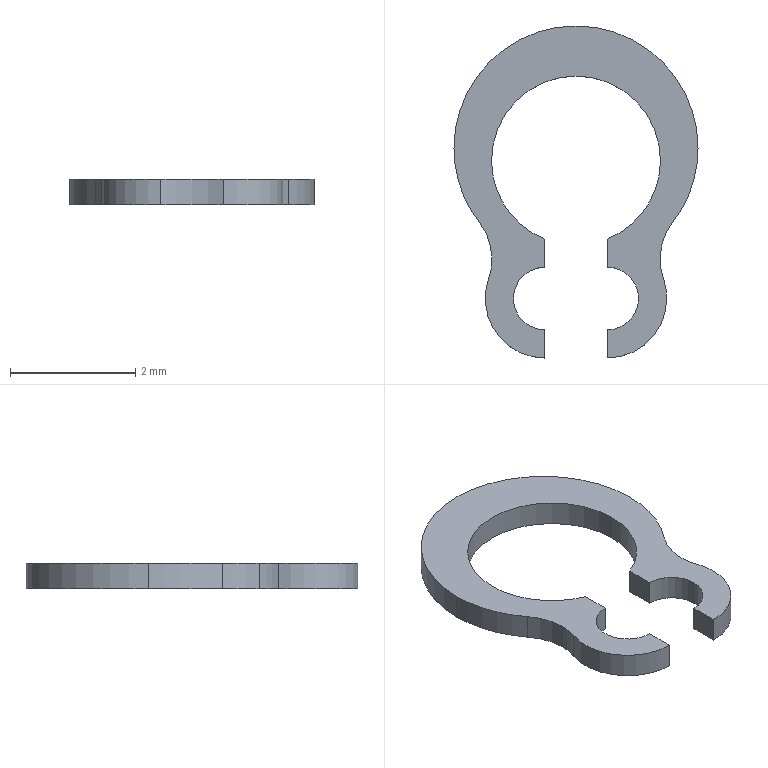Part | SolidWorks | features Boss 1 | 1 solid | 21 faces | box 3.9 x 5.304 x 0.4 mm | volume 3.093 mm3 | cylinder 15 | plane 6 | commonest cylinder face diameters 1.9 x6 1 x3 2.7 x3 3.9 x3
STEP:
#1=CARTESIAN_POINT('',(-0.5,-1.454,-0.4));
#2=VERTEX_POINT('',#1);
#3=CARTESIAN_POINT('',(-1.35,-0.2,-0.4));
#4=VERTEX_POINT('',#3);
#5=CARTESIAN_POINT('',(0.,-0.2,-0.4));
#6=DIRECTION('',(0.,0.,-1.));
#7=DIRECTION('',(1.,0.,0.));
#8=AXIS2_PLACEMENT_3D('',#5,#6,#7);
#9=CIRCLE('',#8,1.35);
#10=EDGE_CURVE('',#2,#4,#9,.T.);
#11=ORIENTED_EDGE('',*,*,#10,.T.);
#12=CARTESIAN_POINT('',(-1.35,-0.2,0.));
#13=VERTEX_POINT('',#12);
#14=CARTESIAN_POINT('',(-1.35,-0.2,-0.4));
#15=DIRECTION('',(0.,0.,1.));
#16=VECTOR('',#15,1000.);
#17=LINE('',#14,#16);
#18=EDGE_CURVE('',#4,#13,#17,.T.);
#19=ORIENTED_EDGE('',*,*,#18,.T.);
#20=CARTESIAN_POINT('',(-0.5,-1.454,0.));
#21=VERTEX_POINT('',#20);
#22=CARTESIAN_POINT('',(0.,-0.2,0.));
#23=DIRECTION('',(0.,0.,-1.));
#24=DIRECTION('',(1.,0.,0.));
#25=AXIS2_PLACEMENT_3D('',#22,#23,#24);
#26=CIRCLE('',#25,1.35);
#27=EDGE_CURVE('',#21,#13,#26,.T.);
#28=ORIENTED_EDGE('',*,*,#27,.F.);
#29=CARTESIAN_POINT('',(-0.5,-1.454,-0.4));
#30=DIRECTION('',(0.,0.,1.));
#31=VECTOR('',#30,1000.);
#32=LINE('',#29,#31);
#33=EDGE_CURVE('',#2,#21,#32,.T.);
#34=ORIENTED_EDGE('',*,*,#33,.F.);
#35=EDGE_LOOP('',(#11,#19,#28,#34));
#36=FACE_OUTER_BOUND('',#35,.T.);
#37=CARTESIAN_POINT('',(0.,-0.2,-0.4));
#38=DIRECTION('',(0.,0.,1.));
#39=DIRECTION('',(1.,0.,0.));
#40=AXIS2_PLACEMENT_3D('',#37,#38,#39);
#41=CYLINDRICAL_SURFACE('',#40,1.35);
#42=ADVANCED_FACE('',(#36),#41,.F.);
#43=ORIENTED_EDGE('',*,*,#18,.F.);
#44=CARTESIAN_POINT('',(1.35,-0.2,-0.4));
#45=VERTEX_POINT('',#44);
#46=CARTESIAN_POINT('',(0.,-0.2,-0.4));
#47=DIRECTION('',(0.,0.,-1.));
#48=DIRECTION('',(1.,0.,0.));
#49=AXIS2_PLACEMENT_3D('',#46,#47,#48);
#50=CIRCLE('',#49,1.35);
#51=EDGE_CURVE('',#4,#45,#50,.T.);
#52=ORIENTED_EDGE('',*,*,#51,.T.);
#53=CARTESIAN_POINT('',(1.35,-0.2,0.));
#54=VERTEX_POINT('',#53);
#55=CARTESIAN_POINT('',(1.35,-0.2,-0.4));
#56=DIRECTION('',(0.,0.,1.));
#57=VECTOR('',#56,1000.);
#58=LINE('',#55,#57);
#59=EDGE_CURVE('',#45,#54,#58,.T.);
#60=ORIENTED_EDGE('',*,*,#59,.T.);
#61=CARTESIAN_POINT('',(0.,-0.2,0.));
#62=DIRECTION('',(0.,0.,-1.));
#63=DIRECTION('',(1.,0.,0.));
#64=AXIS2_PLACEMENT_3D('',#61,#62,#63);
#65=CIRCLE('',#64,1.35);
#66=EDGE_CURVE('',#13,#54,#65,.T.);
#67=ORIENTED_EDGE('',*,*,#66,.F.);
#68=EDGE_LOOP('',(#43,#52,#60,#67));
#69=FACE_OUTER_BOUND('',#68,.T.);
#70=CARTESIAN_POINT('',(0.,-0.2,-0.4));
#71=DIRECTION('',(0.,0.,1.));
#72=DIRECTION('',(1.,0.,0.));
#73=AXIS2_PLACEMENT_3D('',#70,#71,#72);
#74=CYLINDRICAL_SURFACE('',#73,1.35);
#75=ADVANCED_FACE('',(#69),#74,.F.);
#76=CARTESIAN_POINT('',(0.5,-1.904,-0.4));
#77=VERTEX_POINT('',#76);
#78=CARTESIAN_POINT('',(1.,-2.404,-0.4));
#79=VERTEX_POINT('',#78);
#80=CARTESIAN_POINT('',(0.5,-2.404,-0.4));
#81=DIRECTION('',(0.,0.,-1.));
#82=DIRECTION('',(-1.,0.,0.));
#83=AXIS2_PLACEMENT_3D('',#80,#81,#82);
#84=CIRCLE('',#83,0.5);
#85=EDGE_CURVE('',#77,#79,#84,.T.);
#86=ORIENTED_EDGE('',*,*,#85,.T.);
#87=CARTESIAN_POINT('',(1.,-2.404,0.));
#88=VERTEX_POINT('',#87);
#89=CARTESIAN_POINT('',(1.,-2.404,-0.4));
#90=DIRECTION('',(0.,0.,1.));
#91=VECTOR('',#90,1000.);
#92=LINE('',#89,#91);
#93=EDGE_CURVE('',#79,#88,#92,.T.);
#94=ORIENTED_EDGE('',*,*,#93,.T.);
#95=CARTESIAN_POINT('',(0.5,-1.904,0.));
#96=VERTEX_POINT('',#95);
#97=CARTESIAN_POINT('',(0.5,-2.404,0.));
#98=DIRECTION('',(0.,0.,-1.));
#99=DIRECTION('',(-1.,0.,0.));
#100=AXIS2_PLACEMENT_3D('',#97,#98,#99);
#101=CIRCLE('',#100,0.5);
#102=EDGE_CURVE('',#96,#88,#101,.T.);
#103=ORIENTED_EDGE('',*,*,#102,.F.);
#104=CARTESIAN_POINT('',(0.5,-1.904,-0.4));
#105=DIRECTION('',(0.,0.,1.));
#106=VECTOR('',#105,1000.);
#107=LINE('',#104,#106);
#108=EDGE_CURVE('',#77,#96,#107,.T.);
#109=ORIENTED_EDGE('',*,*,#108,.F.);
#110=EDGE_LOOP('',(#86,#94,#103,#109));
#111=FACE_OUTER_BOUND('',#110,.T.);
#112=CARTESIAN_POINT('',(0.5,-2.404,-0.4));
#113=DIRECTION('',(0.,0.,1.));
#114=DIRECTION('',(1.,0.,0.));
#115=AXIS2_PLACEMENT_3D('',#112,#113,#114);
#116=CYLINDRICAL_SURFACE('',#115,0.5);
#117=ADVANCED_FACE('',(#111),#116,.F.);
#118=CARTESIAN_POINT('',(0.5,-3.354,-0.4));
#119=VERTEX_POINT('',#118);
#120=CARTESIAN_POINT('',(1.45,-2.404,-0.4));
#121=VERTEX_POINT('',#120);
#122=CARTESIAN_POINT('',(0.5,-2.404,-0.4));
#123=DIRECTION('',(0.,0.,1.));
#124=DIRECTION('',(1.,0.,0.));
#125=AXIS2_PLACEMENT_3D('',#122,#123,#124);
#126=CIRCLE('',#125,0.95);
#127=EDGE_CURVE('',#119,#121,#126,.T.);
#128=ORIENTED_EDGE('',*,*,#127,.T.);
#129=CARTESIAN_POINT('',(1.45,-2.404,0.));
#130=VERTEX_POINT('',#129);
#131=CARTESIAN_POINT('',(1.45,-2.404,-0.4));
#132=DIRECTION('',(0.,0.,1.));
#133=VECTOR('',#132,1000.);
#134=LINE('',#131,#133);
#135=EDGE_CURVE('',#121,#130,#134,.T.);
#136=ORIENTED_EDGE('',*,*,#135,.T.);
#137=CARTESIAN_POINT('',(0.5,-3.354,0.));
#138=VERTEX_POINT('',#137);
#139=CARTESIAN_POINT('',(0.5,-2.404,0.));
#140=DIRECTION('',(0.,0.,1.));
#141=DIRECTION('',(1.,0.,0.));
#142=AXIS2_PLACEMENT_3D('',#139,#140,#141);
#143=CIRCLE('',#142,0.95);
#144=EDGE_CURVE('',#138,#130,#143,.T.);
#145=ORIENTED_EDGE('',*,*,#144,.F.);
#146=CARTESIAN_POINT('',(0.5,-3.354,-0.4));
#147=DIRECTION('',(0.,0.,1.));
#148=VECTOR('',#147,1000.);
#149=LINE('',#146,#148);
#150=EDGE_CURVE('',#119,#138,#149,.T.);
#151=ORIENTED_EDGE('',*,*,#150,.F.);
#152=EDGE_LOOP('',(#128,#136,#145,#151));
#153=FACE_OUTER_BOUND('',#152,.T.);
#154=CARTESIAN_POINT('',(0.5,-2.404,-0.4));
#155=DIRECTION('',(0.,0.,1.));
#156=DIRECTION('',(1.,0.,0.));
#157=AXIS2_PLACEMENT_3D('',#154,#155,#156);
#158=CYLINDRICAL_SURFACE('',#157,0.95);
#159=ADVANCED_FACE('',(#153),#158,.T.);
#160=CARTESIAN_POINT('',(1.95,0.,-0.4));
#161=VERTEX_POINT('',#160);
#162=CARTESIAN_POINT('',(-1.95,0.,-0.4));
#163=VERTEX_POINT('',#162);
#164=CARTESIAN_POINT('',(0.,0.,-0.4));
#165=DIRECTION('',(0.,0.,1.));
#166=DIRECTION('',(1.,0.,0.));
#167=AXIS2_PLACEMENT_3D('',#164,#165,#166);
#168=CIRCLE('',#167,1.95);
#169=EDGE_CURVE('',#161,#163,#168,.T.);
#170=ORIENTED_EDGE('',*,*,#169,.T.);
#171=CARTESIAN_POINT('',(-1.95,0.,0.));
#172=VERTEX_POINT('',#171);
#173=CARTESIAN_POINT('',(-1.95,0.,-0.4));
#174=DIRECTION('',(0.,0.,1.));
#175=VECTOR('',#174,1000.);
#176=LINE('',#173,#175);
#177=EDGE_CURVE('',#163,#172,#176,.T.);
#178=ORIENTED_EDGE('',*,*,#177,.T.);
#179=CARTESIAN_POINT('',(1.95,0.,0.));
#180=VERTEX_POINT('',#179);
#181=CARTESIAN_POINT('',(0.,0.,0.));
#182=DIRECTION('',(0.,0.,1.));
#183=DIRECTION('',(1.,0.,0.));
#184=AXIS2_PLACEMENT_3D('',#181,#182,#183);
#185=CIRCLE('',#184,1.95);
#186=EDGE_CURVE('',#180,#172,#185,.T.);
#187=ORIENTED_EDGE('',*,*,#186,.F.);
#188=CARTESIAN_POINT('',(1.95,0.,-0.4));
#189=DIRECTION('',(0.,0.,1.));
#190=VECTOR('',#189,1000.);
#191=LINE('',#188,#190);
#192=EDGE_CURVE('',#161,#180,#191,.T.);
#193=ORIENTED_EDGE('',*,*,#192,.F.);
#194=EDGE_LOOP('',(#170,#178,#187,#193));
#195=FACE_OUTER_BOUND('',#194,.T.);
#196=CARTESIAN_POINT('',(0.,0.,-0.4));
#197=DIRECTION('',(0.,0.,1.));
#198=DIRECTION('',(1.,0.,0.));
#199=AXIS2_PLACEMENT_3D('',#196,#197,#198);
#200=CYLINDRICAL_SURFACE('',#199,1.95);
#201=ADVANCED_FACE('',(#195),#200,.T.);
#202=CARTESIAN_POINT('',(1.542,-1.194,-0.4));
#203=VERTEX_POINT('',#202);
#204=CARTESIAN_POINT('',(0.,0.,-0.4));
#205=DIRECTION('',(0.,0.,1.));
#206=DIRECTION('',(1.,0.,0.));
#207=AXIS2_PLACEMENT_3D('',#204,#205,#206);
#208=CIRCLE('',#207,1.95);
#209=EDGE_CURVE('',#203,#161,#208,.T.);
#210=ORIENTED_EDGE('',*,*,#209,.T.);
#211=ORIENTED_EDGE('',*,*,#192,.T.);
#212=CARTESIAN_POINT('',(1.542,-1.194,0.));
#213=VERTEX_POINT('',#212);
#214=CARTESIAN_POINT('',(0.,0.,0.));
#215=DIRECTION('',(0.,0.,1.));
#216=DIRECTION('',(1.,0.,0.));
#217=AXIS2_PLACEMENT_3D('',#214,#215,#216);
#218=CIRCLE('',#217,1.95);
#219=EDGE_CURVE('',#213,#180,#218,.T.);
#220=ORIENTED_EDGE('',*,*,#219,.F.);
#221=CARTESIAN_POINT('',(1.542,-1.194,-0.4));
#222=DIRECTION('',(0.,0.,1.));
#223=VECTOR('',#222,1000.);
#224=LINE('',#221,#223);
#225=EDGE_CURVE('',#203,#213,#224,.T.);
#226=ORIENTED_EDGE('',*,*,#225,.F.);
#227=EDGE_LOOP('',(#210,#211,#220,#226));
#228=FACE_OUTER_BOUND('',#227,.T.);
#229=CARTESIAN_POINT('',(0.,0.,-0.4));
#230=DIRECTION('',(0.,0.,1.));
#231=DIRECTION('',(1.,0.,0.));
#232=AXIS2_PLACEMENT_3D('',#229,#230,#231);
#233=CYLINDRICAL_SURFACE('',#232,1.95);
#234=ADVANCED_FACE('',(#228),#233,.T.);
#235=CARTESIAN_POINT('',(-1.542,-1.194,-0.4));
#236=VERTEX_POINT('',#235);
#237=CARTESIAN_POINT('',(-1.343,-1.775,-0.4));
#238=VERTEX_POINT('',#237);
#239=CARTESIAN_POINT('',(-2.293,-1.775,-0.4));
#240=DIRECTION('',(0.,0.,-1.));
#241=DIRECTION('',(-1.,0.,0.));
#242=AXIS2_PLACEMENT_3D('',#239,#240,#241);
#243=CIRCLE('',#242,0.95);
#244=EDGE_CURVE('',#236,#238,#243,.T.);
#245=ORIENTED_EDGE('',*,*,#244,.T.);
#246=CARTESIAN_POINT('',(-1.343,-1.775,0.));
#247=VERTEX_POINT('',#246);
#248=CARTESIAN_POINT('',(-1.343,-1.775,-0.4));
#249=DIRECTION('',(0.,0.,1.));
#250=VECTOR('',#249,1000.);
#251=LINE('',#248,#250);
#252=EDGE_CURVE('',#238,#247,#251,.T.);
#253=ORIENTED_EDGE('',*,*,#252,.T.);
#254=CARTESIAN_POINT('',(-1.542,-1.194,0.));
#255=VERTEX_POINT('',#254);
#256=CARTESIAN_POINT('',(-2.293,-1.775,0.));
#257=DIRECTION('',(0.,0.,-1.));
#258=DIRECTION('',(-1.,0.,0.));
#259=AXIS2_PLACEMENT_3D('',#256,#257,#258);
#260=CIRCLE('',#259,0.95);
#261=EDGE_CURVE('',#255,#247,#260,.T.);
#262=ORIENTED_EDGE('',*,*,#261,.F.);
#263=CARTESIAN_POINT('',(-1.542,-1.194,-0.4));
#264=DIRECTION('',(0.,0.,1.));
#265=VECTOR('',#264,1000.);
#266=LINE('',#263,#265);
#267=EDGE_CURVE('',#236,#255,#266,.T.);
#268=ORIENTED_EDGE('',*,*,#267,.F.);
#269=EDGE_LOOP('',(#245,#253,#262,#268));
#270=FACE_OUTER_BOUND('',#269,.T.);
#271=CARTESIAN_POINT('',(-2.293,-1.775,-0.4));
#272=DIRECTION('',(0.,0.,1.));
#273=DIRECTION('',(1.,0.,0.));
#274=AXIS2_PLACEMENT_3D('',#271,#272,#273);
#275=CYLINDRICAL_SURFACE('',#274,0.95);
#276=ADVANCED_FACE('',(#270),#275,.F.);
#277=CARTESIAN_POINT('',(-0.5,-2.904,0.));
#278=VERTEX_POINT('',#277);
#279=CARTESIAN_POINT('',(-0.5,-1.904,0.));
#280=VERTEX_POINT('',#279);
#281=CARTESIAN_POINT('',(-0.5,-2.404,0.));
#282=DIRECTION('',(0.,0.,-1.));
#283=DIRECTION('',(1.,0.,0.));
#284=AXIS2_PLACEMENT_3D('',#281,#282,#283);
#285=CIRCLE('',#284,0.5);
#286=EDGE_CURVE('',#278,#280,#285,.T.);
#287=ORIENTED_EDGE('',*,*,#286,.F.);
#288=CARTESIAN_POINT('',(-0.5,-2.904,-0.4));
#289=VERTEX_POINT('',#288);
#290=CARTESIAN_POINT('',(-0.5,-2.904,-0.4));
#291=DIRECTION('',(0.,0.,1.));
#292=VECTOR('',#291,1000.);
#293=LINE('',#290,#292);
#294=EDGE_CURVE('',#289,#278,#293,.T.);
#295=ORIENTED_EDGE('',*,*,#294,.F.);
#296=CARTESIAN_POINT('',(-0.5,-1.904,-0.4));
#297=VERTEX_POINT('',#296);
#298=CARTESIAN_POINT('',(-0.5,-2.404,-0.4));
#299=DIRECTION('',(0.,0.,-1.));
#300=DIRECTION('',(1.,0.,0.));
#301=AXIS2_PLACEMENT_3D('',#298,#299,#300);
#302=CIRCLE('',#301,0.5);
#303=EDGE_CURVE('',#289,#297,#302,.T.);
#304=ORIENTED_EDGE('',*,*,#303,.T.);
#305=CARTESIAN_POINT('',(-0.5,-1.904,-0.4));
#306=DIRECTION('',(0.,0.,1.));
#307=VECTOR('',#306,1000.);
#308=LINE('',#305,#307);
#309=EDGE_CURVE('',#297,#280,#308,.T.);
#310=ORIENTED_EDGE('',*,*,#309,.T.);
#311=EDGE_LOOP('',(#287,#295,#304,#310));
#312=FACE_OUTER_BOUND('',#311,.T.);
#313=CARTESIAN_POINT('',(-0.5,-2.404,-0.4));
#314=DIRECTION('',(0.,0.,1.));
#315=DIRECTION('',(1.,0.,0.));
#316=AXIS2_PLACEMENT_3D('',#313,#314,#315);
#317=CYLINDRICAL_SURFACE('',#316,0.5);
#318=ADVANCED_FACE('',(#312),#317,.F.);
#319=CARTESIAN_POINT('',(-0.5,-3.354,0.));
#320=VERTEX_POINT('',#319);
#321=CARTESIAN_POINT('',(-0.5,-2.904,0.));
#322=DIRECTION('',(0.,1.,0.));
#323=VECTOR('',#322,1000.);
#324=LINE('',#321,#323);
#325=EDGE_CURVE('',#320,#278,#324,.T.);
#326=ORIENTED_EDGE('',*,*,#325,.F.);
#327=CARTESIAN_POINT('',(-0.5,-3.354,-0.4));
#328=VERTEX_POINT('',#327);
#329=CARTESIAN_POINT('',(-0.5,-3.354,-0.4));
#330=DIRECTION('',(0.,0.,1.));
#331=VECTOR('',#330,1000.);
#332=LINE('',#329,#331);
#333=EDGE_CURVE('',#328,#320,#332,.T.);
#334=ORIENTED_EDGE('',*,*,#333,.F.);
#335=CARTESIAN_POINT('',(-0.5,-2.904,-0.4));
#336=DIRECTION('',(0.,1.,0.));
#337=VECTOR('',#336,1000.);
#338=LINE('',#335,#337);
#339=EDGE_CURVE('',#328,#289,#338,.T.);
#340=ORIENTED_EDGE('',*,*,#339,.T.);
#341=ORIENTED_EDGE('',*,*,#294,.T.);
#342=EDGE_LOOP('',(#326,#334,#340,#341));
#343=FACE_OUTER_BOUND('',#342,.T.);
#344=CARTESIAN_POINT('',(-0.5,-2.904,-0.4));
#345=DIRECTION('',(1.,0.,0.));
#346=DIRECTION('',(0.,0.,-1.));
#347=AXIS2_PLACEMENT_3D('',#344,#345,#346);
#348=PLANE('',#347);
#349=ADVANCED_FACE('',(#343),#348,.T.);
#350=CARTESIAN_POINT('',(-1.397,-2.09,0.));
#351=VERTEX_POINT('',#350);
#352=CARTESIAN_POINT('',(-0.5,-2.404,0.));
#353=DIRECTION('',(0.,0.,1.));
#354=DIRECTION('',(-1.,0.,0.));
#355=AXIS2_PLACEMENT_3D('',#352,#353,#354);
#356=CIRCLE('',#355,0.95);
#357=EDGE_CURVE('',#351,#320,#356,.T.);
#358=ORIENTED_EDGE('',*,*,#357,.F.);
#359=CARTESIAN_POINT('',(-1.397,-2.09,-0.4));
#360=VERTEX_POINT('',#359);
#361=CARTESIAN_POINT('',(-1.397,-2.09,-0.4));
#362=DIRECTION('',(0.,0.,1.));
#363=VECTOR('',#362,1000.);
#364=LINE('',#361,#363);
#365=EDGE_CURVE('',#360,#351,#364,.T.);
#366=ORIENTED_EDGE('',*,*,#365,.F.);
#367=CARTESIAN_POINT('',(-0.5,-2.404,-0.4));
#368=DIRECTION('',(0.,0.,1.));
#369=DIRECTION('',(-1.,0.,0.));
#370=AXIS2_PLACEMENT_3D('',#367,#368,#369);
#371=CIRCLE('',#370,0.95);
#372=EDGE_CURVE('',#360,#328,#371,.T.);
#373=ORIENTED_EDGE('',*,*,#372,.T.);
#374=ORIENTED_EDGE('',*,*,#333,.T.);
#375=EDGE_LOOP('',(#358,#366,#373,#374));
#376=FACE_OUTER_BOUND('',#375,.T.);
#377=CARTESIAN_POINT('',(-0.5,-2.404,-0.4));
#378=DIRECTION('',(0.,0.,1.));
#379=DIRECTION('',(1.,0.,0.));
#380=AXIS2_PLACEMENT_3D('',#377,#378,#379);
#381=CYLINDRICAL_SURFACE('',#380,0.95);
#382=ADVANCED_FACE('',(#376),#381,.T.);
#383=ORIENTED_EDGE('',*,*,#252,.F.);
#384=CARTESIAN_POINT('',(-2.293,-1.775,-0.4));
#385=DIRECTION('',(0.,0.,-1.));
#386=DIRECTION('',(-1.,0.,0.));
#387=AXIS2_PLACEMENT_3D('',#384,#385,#386);
#388=CIRCLE('',#387,0.95);
#389=EDGE_CURVE('',#238,#360,#388,.T.);
#390=ORIENTED_EDGE('',*,*,#389,.T.);
#391=ORIENTED_EDGE('',*,*,#365,.T.);
#392=CARTESIAN_POINT('',(-2.293,-1.775,0.));
#393=DIRECTION('',(0.,0.,-1.));
#394=DIRECTION('',(-1.,0.,0.));
#395=AXIS2_PLACEMENT_3D('',#392,#393,#394);
#396=CIRCLE('',#395,0.95);
#397=EDGE_CURVE('',#247,#351,#396,.T.);
#398=ORIENTED_EDGE('',*,*,#397,.F.);
#399=EDGE_LOOP('',(#383,#390,#391,#398));
#400=FACE_OUTER_BOUND('',#399,.T.);
#401=CARTESIAN_POINT('',(-2.293,-1.775,-0.4));
#402=DIRECTION('',(0.,0.,1.));
#403=DIRECTION('',(1.,0.,0.));
#404=AXIS2_PLACEMENT_3D('',#401,#402,#403);
#405=CYLINDRICAL_SURFACE('',#404,0.95);
#406=ADVANCED_FACE('',(#400),#405,.F.);
#407=ORIENTED_EDGE('',*,*,#177,.F.);
#408=CARTESIAN_POINT('',(0.,0.,-0.4));
#409=DIRECTION('',(0.,0.,1.));
#410=DIRECTION('',(1.,0.,0.));
#411=AXIS2_PLACEMENT_3D('',#408,#409,#410);
#412=CIRCLE('',#411,1.95);
#413=EDGE_CURVE('',#163,#236,#412,.T.);
#414=ORIENTED_EDGE('',*,*,#413,.T.);
#415=ORIENTED_EDGE('',*,*,#267,.T.);
#416=CARTESIAN_POINT('',(0.,0.,0.));
#417=DIRECTION('',(0.,0.,1.));
#418=DIRECTION('',(1.,0.,0.));
#419=AXIS2_PLACEMENT_3D('',#416,#417,#418);
#420=CIRCLE('',#419,1.95);
#421=EDGE_CURVE('',#172,#255,#420,.T.);
#422=ORIENTED_EDGE('',*,*,#421,.F.);
#423=EDGE_LOOP('',(#407,#414,#415,#422));
#424=FACE_OUTER_BOUND('',#423,.T.);
#425=CARTESIAN_POINT('',(0.,0.,-0.4));
#426=DIRECTION('',(0.,0.,1.));
#427=DIRECTION('',(1.,0.,0.));
#428=AXIS2_PLACEMENT_3D('',#425,#426,#427);
#429=CYLINDRICAL_SURFACE('',#428,1.95);
#430=ADVANCED_FACE('',(#424),#429,.T.);
#431=CARTESIAN_POINT('',(1.397,-2.09,0.));
#432=VERTEX_POINT('',#431);
#433=CARTESIAN_POINT('',(2.293,-1.775,0.));
#434=DIRECTION('',(0.,0.,-1.));
#435=DIRECTION('',(1.,0.,0.));
#436=AXIS2_PLACEMENT_3D('',#433,#434,#435);
#437=CIRCLE('',#436,0.95);
#438=EDGE_CURVE('',#432,#213,#437,.T.);
#439=ORIENTED_EDGE('',*,*,#438,.F.);
#440=CARTESIAN_POINT('',(1.397,-2.09,-0.4));
#441=VERTEX_POINT('',#440);
#442=CARTESIAN_POINT('',(1.397,-2.09,-0.4));
#443=DIRECTION('',(0.,0.,1.));
#444=VECTOR('',#443,1000.);
#445=LINE('',#442,#444);
#446=EDGE_CURVE('',#441,#432,#445,.T.);
#447=ORIENTED_EDGE('',*,*,#446,.F.);
#448=CARTESIAN_POINT('',(2.293,-1.775,-0.4));
#449=DIRECTION('',(0.,0.,-1.));
#450=DIRECTION('',(1.,0.,0.));
#451=AXIS2_PLACEMENT_3D('',#448,#449,#450);
#452=CIRCLE('',#451,0.95);
#453=EDGE_CURVE('',#441,#203,#452,.T.);
#454=ORIENTED_EDGE('',*,*,#453,.T.);
#455=ORIENTED_EDGE('',*,*,#225,.T.);
#456=EDGE_LOOP('',(#439,#447,#454,#455));
#457=FACE_OUTER_BOUND('',#456,.T.);
#458=CARTESIAN_POINT('',(2.293,-1.775,-0.4));
#459=DIRECTION('',(0.,0.,1.));
#460=DIRECTION('',(1.,0.,0.));
#461=AXIS2_PLACEMENT_3D('',#458,#459,#460);
#462=CYLINDRICAL_SURFACE('',#461,0.95);
#463=ADVANCED_FACE('',(#457),#462,.F.);
#464=ORIENTED_EDGE('',*,*,#135,.F.);
#465=CARTESIAN_POINT('',(0.5,-2.404,-0.4));
#466=DIRECTION('',(0.,0.,1.));
#467=DIRECTION('',(1.,0.,0.));
#468=AXIS2_PLACEMENT_3D('',#465,#466,#467);
#469=CIRCLE('',#468,0.95);
#470=EDGE_CURVE('',#121,#441,#469,.T.);
#471=ORIENTED_EDGE('',*,*,#470,.T.);
#472=ORIENTED_EDGE('',*,*,#446,.T.);
#473=CARTESIAN_POINT('',(0.5,-2.404,0.));
#474=DIRECTION('',(0.,0.,1.));
#475=DIRECTION('',(1.,0.,0.));
#476=AXIS2_PLACEMENT_3D('',#473,#474,#475);
#477=CIRCLE('',#476,0.95);
#478=EDGE_CURVE('',#130,#432,#477,.T.);
#479=ORIENTED_EDGE('',*,*,#478,.F.);
#480=EDGE_LOOP('',(#464,#471,#472,#479));
#481=FACE_OUTER_BOUND('',#480,.T.);
#482=CARTESIAN_POINT('',(0.5,-2.404,-0.4));
#483=DIRECTION('',(0.,0.,1.));
#484=DIRECTION('',(1.,0.,0.));
#485=AXIS2_PLACEMENT_3D('',#482,#483,#484);
#486=CYLINDRICAL_SURFACE('',#485,0.95);
#487=ADVANCED_FACE('',(#481),#486,.T.);
#488=CARTESIAN_POINT('',(0.5,-2.904,0.));
#489=VERTEX_POINT('',#488);
#490=CARTESIAN_POINT('',(0.5,-2.904,0.));
#491=DIRECTION('',(0.,-1.,0.));
#492=VECTOR('',#491,1000.);
#493=LINE('',#490,#492);
#494=EDGE_CURVE('',#489,#138,#493,.T.);
#495=ORIENTED_EDGE('',*,*,#494,.F.);
#496=CARTESIAN_POINT('',(0.5,-2.904,-0.4));
#497=VERTEX_POINT('',#496);
#498=CARTESIAN_POINT('',(0.5,-2.904,-0.4));
#499=DIRECTION('',(0.,0.,1.));
#500=VECTOR('',#499,1000.);
#501=LINE('',#498,#500);
#502=EDGE_CURVE('',#497,#489,#501,.T.);
#503=ORIENTED_EDGE('',*,*,#502,.F.);
#504=CARTESIAN_POINT('',(0.5,-2.904,-0.4));
#505=DIRECTION('',(0.,-1.,0.));
#506=VECTOR('',#505,1000.);
#507=LINE('',#504,#506);
#508=EDGE_CURVE('',#497,#119,#507,.T.);
#509=ORIENTED_EDGE('',*,*,#508,.T.);
#510=ORIENTED_EDGE('',*,*,#150,.T.);
#511=EDGE_LOOP('',(#495,#503,#509,#510));
#512=FACE_OUTER_BOUND('',#511,.T.);
#513=CARTESIAN_POINT('',(0.5,-2.904,-0.4));
#514=DIRECTION('',(-1.,0.,0.));
#515=DIRECTION('',(0.,0.,1.));
#516=AXIS2_PLACEMENT_3D('',#513,#514,#515);
#517=PLANE('',#516);
#518=ADVANCED_FACE('',(#512),#517,.T.);
#519=ORIENTED_EDGE('',*,*,#93,.F.);
#520=CARTESIAN_POINT('',(0.5,-2.404,-0.4));
#521=DIRECTION('',(0.,0.,-1.));
#522=DIRECTION('',(-1.,0.,0.));
#523=AXIS2_PLACEMENT_3D('',#520,#521,#522);
#524=CIRCLE('',#523,0.5);
#525=EDGE_CURVE('',#79,#497,#524,.T.);
#526=ORIENTED_EDGE('',*,*,#525,.T.);
#527=ORIENTED_EDGE('',*,*,#502,.T.);
#528=CARTESIAN_POINT('',(0.5,-2.404,0.));
#529=DIRECTION('',(0.,0.,-1.));
#530=DIRECTION('',(-1.,0.,0.));
#531=AXIS2_PLACEMENT_3D('',#528,#529,#530);
#532=CIRCLE('',#531,0.5);
#533=EDGE_CURVE('',#88,#489,#532,.T.);
#534=ORIENTED_EDGE('',*,*,#533,.F.);
#535=EDGE_LOOP('',(#519,#526,#527,#534));
#536=FACE_OUTER_BOUND('',#535,.T.);
#537=CARTESIAN_POINT('',(0.5,-2.404,-0.4));
#538=DIRECTION('',(0.,0.,1.));
#539=DIRECTION('',(1.,0.,0.));
#540=AXIS2_PLACEMENT_3D('',#537,#538,#539);
#541=CYLINDRICAL_SURFACE('',#540,0.5);
#542=ADVANCED_FACE('',(#536),#541,.F.);
#543=CARTESIAN_POINT('',(0.5,-1.454,0.));
#544=VERTEX_POINT('',#543);
#545=CARTESIAN_POINT('',(0.5,-1.454,0.));
#546=DIRECTION('',(0.,-1.,0.));
#547=VECTOR('',#546,1000.);
#548=LINE('',#545,#547);
#549=EDGE_CURVE('',#544,#96,#548,.T.);
#550=ORIENTED_EDGE('',*,*,#549,.F.);
#551=CARTESIAN_POINT('',(0.5,-1.454,-0.4));
#552=VERTEX_POINT('',#551);
#553=CARTESIAN_POINT('',(0.5,-1.454,-0.4));
#554=DIRECTION('',(0.,0.,1.));
#555=VECTOR('',#554,1000.);
#556=LINE('',#553,#555);
#557=EDGE_CURVE('',#552,#544,#556,.T.);
#558=ORIENTED_EDGE('',*,*,#557,.F.);
#559=CARTESIAN_POINT('',(0.5,-1.454,-0.4));
#560=DIRECTION('',(0.,-1.,0.));
#561=VECTOR('',#560,1000.);
#562=LINE('',#559,#561);
#563=EDGE_CURVE('',#552,#77,#562,.T.);
#564=ORIENTED_EDGE('',*,*,#563,.T.);
#565=ORIENTED_EDGE('',*,*,#108,.T.);
#566=EDGE_LOOP('',(#550,#558,#564,#565));
#567=FACE_OUTER_BOUND('',#566,.T.);
#568=CARTESIAN_POINT('',(0.5,-1.454,-0.4));
#569=DIRECTION('',(-1.,0.,0.));
#570=DIRECTION('',(0.,-1.,0.));
#571=AXIS2_PLACEMENT_3D('',#568,#569,#570);
#572=PLANE('',#571);
#573=ADVANCED_FACE('',(#567),#572,.T.);
#574=ORIENTED_EDGE('',*,*,#59,.F.);
#575=CARTESIAN_POINT('',(0.,-0.2,-0.4));
#576=DIRECTION('',(0.,0.,-1.));
#577=DIRECTION('',(1.,0.,0.));
#578=AXIS2_PLACEMENT_3D('',#575,#576,#577);
#579=CIRCLE('',#578,1.35);
#580=EDGE_CURVE('',#45,#552,#579,.T.);
#581=ORIENTED_EDGE('',*,*,#580,.T.);
#582=ORIENTED_EDGE('',*,*,#557,.T.);
#583=CARTESIAN_POINT('',(0.,-0.2,0.));
#584=DIRECTION('',(0.,0.,-1.));
#585=DIRECTION('',(1.,0.,0.));
#586=AXIS2_PLACEMENT_3D('',#583,#584,#585);
#587=CIRCLE('',#586,1.35);
#588=EDGE_CURVE('',#54,#544,#587,.T.);
#589=ORIENTED_EDGE('',*,*,#588,.F.);
#590=EDGE_LOOP('',(#574,#581,#582,#589));
#591=FACE_OUTER_BOUND('',#590,.T.);
#592=CARTESIAN_POINT('',(0.,-0.2,-0.4));
#593=DIRECTION('',(0.,0.,1.));
#594=DIRECTION('',(1.,0.,0.));
#595=AXIS2_PLACEMENT_3D('',#592,#593,#594);
#596=CYLINDRICAL_SURFACE('',#595,1.35);
#597=ADVANCED_FACE('',(#591),#596,.F.);
#598=CARTESIAN_POINT('',(-0.5,-1.454,0.));
#599=DIRECTION('',(0.,1.,0.));
#600=VECTOR('',#599,1000.);
#601=LINE('',#598,#600);
#602=EDGE_CURVE('',#280,#21,#601,.T.);
#603=ORIENTED_EDGE('',*,*,#602,.F.);
#604=ORIENTED_EDGE('',*,*,#309,.F.);
#605=CARTESIAN_POINT('',(-0.5,-1.454,-0.4));
#606=DIRECTION('',(0.,1.,0.));
#607=VECTOR('',#606,1000.);
#608=LINE('',#605,#607);
#609=EDGE_CURVE('',#297,#2,#608,.T.);
#610=ORIENTED_EDGE('',*,*,#609,.T.);
#611=ORIENTED_EDGE('',*,*,#33,.T.);
#612=EDGE_LOOP('',(#603,#604,#610,#611));
#613=FACE_OUTER_BOUND('',#612,.T.);
#614=CARTESIAN_POINT('',(-0.5,-1.454,-0.4));
#615=DIRECTION('',(1.,0.,0.));
#616=DIRECTION('',(0.,1.,0.));
#617=AXIS2_PLACEMENT_3D('',#614,#615,#616);
#618=PLANE('',#617);
#619=ADVANCED_FACE('',(#613),#618,.T.);
#620=ORIENTED_EDGE('',*,*,#303,.F.);
#621=ORIENTED_EDGE('',*,*,#339,.F.);
#622=ORIENTED_EDGE('',*,*,#372,.F.);
#623=ORIENTED_EDGE('',*,*,#389,.F.);
#624=ORIENTED_EDGE('',*,*,#244,.F.);
#625=ORIENTED_EDGE('',*,*,#413,.F.);
#626=ORIENTED_EDGE('',*,*,#169,.F.);
#627=ORIENTED_EDGE('',*,*,#209,.F.);
#628=ORIENTED_EDGE('',*,*,#453,.F.);
#629=ORIENTED_EDGE('',*,*,#470,.F.);
#630=ORIENTED_EDGE('',*,*,#127,.F.);
#631=ORIENTED_EDGE('',*,*,#508,.F.);
#632=ORIENTED_EDGE('',*,*,#525,.F.);
#633=ORIENTED_EDGE('',*,*,#85,.F.);
#634=ORIENTED_EDGE('',*,*,#563,.F.);
#635=ORIENTED_EDGE('',*,*,#580,.F.);
#636=ORIENTED_EDGE('',*,*,#51,.F.);
#637=ORIENTED_EDGE('',*,*,#10,.F.);
#638=ORIENTED_EDGE('',*,*,#609,.F.);
#639=EDGE_LOOP('',(#620,#621,#622,#623,#624,#625,#626,#627,#628,#629,#630,#631,#632,#633,#634,#635,#636,#637,#638));
#640=FACE_OUTER_BOUND('',#639,.T.);
#641=CARTESIAN_POINT('',(-0.5,-2.404,-0.4));
#642=DIRECTION('',(0.,0.,1.));
#643=DIRECTION('',(1.,0.,0.));
#644=AXIS2_PLACEMENT_3D('',#641,#642,#643);
#645=PLANE('',#644);
#646=ADVANCED_FACE('',(#640),#645,.F.);
#647=ORIENTED_EDGE('',*,*,#286,.T.);
#648=ORIENTED_EDGE('',*,*,#602,.T.);
#649=ORIENTED_EDGE('',*,*,#27,.T.);
#650=ORIENTED_EDGE('',*,*,#66,.T.);
#651=ORIENTED_EDGE('',*,*,#588,.T.);
#652=ORIENTED_EDGE('',*,*,#549,.T.);
#653=ORIENTED_EDGE('',*,*,#102,.T.);
#654=ORIENTED_EDGE('',*,*,#533,.T.);
#655=ORIENTED_EDGE('',*,*,#494,.T.);
#656=ORIENTED_EDGE('',*,*,#144,.T.);
#657=ORIENTED_EDGE('',*,*,#478,.T.);
#658=ORIENTED_EDGE('',*,*,#438,.T.);
#659=ORIENTED_EDGE('',*,*,#219,.T.);
#660=ORIENTED_EDGE('',*,*,#186,.T.);
#661=ORIENTED_EDGE('',*,*,#421,.T.);
#662=ORIENTED_EDGE('',*,*,#261,.T.);
#663=ORIENTED_EDGE('',*,*,#397,.T.);
#664=ORIENTED_EDGE('',*,*,#357,.T.);
#665=ORIENTED_EDGE('',*,*,#325,.T.);
#666=EDGE_LOOP('',(#647,#648,#649,#650,#651,#652,#653,#654,#655,#656,#657,#658,#659,#660,#661,#662,#663,#664,#665));
#667=FACE_OUTER_BOUND('',#666,.T.);
#668=CARTESIAN_POINT('',(-0.5,-2.404,0.));
#669=DIRECTION('',(0.,0.,1.));
#670=DIRECTION('',(1.,0.,0.));
#671=AXIS2_PLACEMENT_3D('',#668,#669,#670);
#672=PLANE('',#671);
#673=ADVANCED_FACE('',(#667),#672,.T.);
#674=CLOSED_SHELL('',(#42,#75,#117,#159,#201,#234,#276,#318,#349,#382,#406,#430,#463,#487,#518,#542,#573,#597,#619,#646,#673));
#675=MANIFOLD_SOLID_BREP('',#674);
#676=CARTESIAN_POINT('',(0.,0.,0.));
#677=DIRECTION('',(0.,0.,1.));
#678=DIRECTION('',(1.,0.,0.));
#679=AXIS2_PLACEMENT_3D('',#676,#677,#678);
#680=(LENGTH_UNIT()NAMED_UNIT(*)SI_UNIT(.MILLI.,.METRE.));
#681=UNCERTAINTY_MEASURE_WITH_UNIT(LENGTH_MEASURE(0.00001),#680,'','');
#682=(NAMED_UNIT(*)PLANE_ANGLE_UNIT()SI_UNIT($,.RADIAN.));
#683=(NAMED_UNIT(*)SI_UNIT($,.STERADIAN.)SOLID_ANGLE_UNIT());
#684=(GEOMETRIC_REPRESENTATION_CONTEXT(3)GLOBAL_UNCERTAINTY_ASSIGNED_CONTEXT((#681))GLOBAL_UNIT_ASSIGNED_CONTEXT((#680,#682,#683))REPRESENTATION_CONTEXT('',''));
#685=ADVANCED_BREP_SHAPE_REPRESENTATION('',(#675,#679),#684);